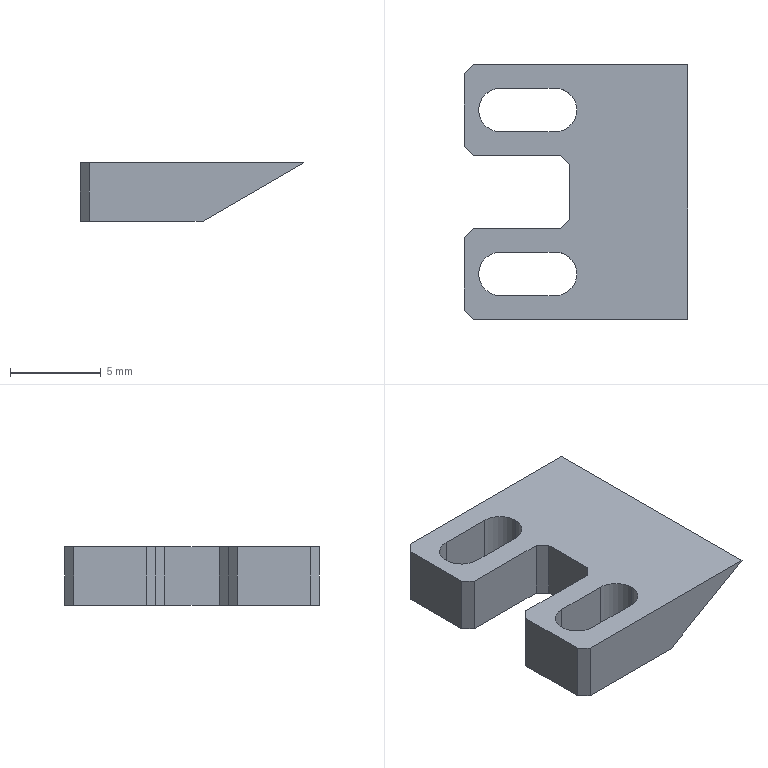NC program | NX | posted with a generic post | part box 12.3 x 14 x 3.2 mm
Whole program:
N10 G17 G21 G94 G90
(FLOOR_WALL , TOOL : D10JING)
N12 T09 M6
N14 G54
N16 G17 G0 G90 X17. Y-8.147 S9500 M3
N18 G43 Z30. H9
N20 Z3.
N22 G94 G1 Z0. F1250.
N24 X14.
N26 X-14.
N28 Y-4.048
N30 X14.
N32 Y0.051
N34 X-14.
N36 Y4.15
N38 X14.
N40 X17.
N42 Z3.
N44 G0 Z30.
N46 M5
(ZLEVEL_PROFILE , TOOL : D6)
N48 T06 M6
N50 G54
N52 G17 G0 G90 X-10.1 Y5.695 S9500 M3
N54 G43 Z30. H6
N56 Z1.5
N58 G94 G1 Y6.082 Z1.48 F1000.
N60 X-9.903 Y6.82 Z1.44
N62 X-9.534 Y7.488 Z1.4
N64 X-9.192 Y7.842 Z1.374
N66 X-8.692 Y8.342 Z1.337
N68 X-8.386 Y8.648 Z1.314
N70 X-7.698 Y9.042 Z1.273
N72 X-6.932 Y9.25 Z1.231
N74 X-2.068 Z0.976
N76 X-1.302 Y9.042 Z0.935
N78 X-0.614 Y8.648 Z0.893
N80 X-0.308 Y8.342 Z0.87
N82 X-0.001 Y8.033 Z0.847
N84 X0.614 Y8.648 Z0.802
N86 X1.302 Y9.042 Z0.76
N88 X2.068 Y9.25 Z0.719
N90 X6.932 Z0.464
N92 X7.672 Y9.052 Z0.424
N94 X8.341 Y8.681 Z0.384
N96 X8.692 Y8.342 Z0.358
N98 X9.192 Y7.842 Z0.321
N100 X9.498 Y7.536 Z0.298
N102 X9.892 Y6.848 Z0.257
N104 X10.1 Y6.082 Z0.215
N106 Y-1.362 Z-0.175
N108 X10.107 Y-1.798 Z-0.198
N110 X9.82 Y-2.783 Z-0.252
N112 X9.234 Y-3.625 Z-0.305
N114 X8.411 Y-4.237 Z-0.359
N116 X7.436 Y-4.555 Z-0.413
N118 X7. Y-4.562 Z-0.436
N120 X-7. F2500.
N122 G2 X-10.1 Y-1.362 R3.181
N124 G1 Y5.65
N126 G2 X-9.192 Y7.842 R3.1
N128 G1 X-8.692 Y8.342
N130 G2 X-6.5 Y9.25 R3.1
N132 G1 X-2.5
N134 G2 X-0.308 Y8.342 R3.1
N136 G1 X-0.001 Y8.033
N138 X0.308 Y8.342
N140 G2 X2.5 Y9.25 R3.1
N142 G1 X6.5
N144 G2 X8.692 Y8.342 R3.1
N146 G1 X9.192 Y7.842
N148 G2 X10.1 Y5.65 R3.1
N150 G1 Y-1.362
N152 G2 X7. Y-4.562 R3.15
N154 G1 X-6.67 Y-4.975 Z-0.674
N156 X-6.99 Y-4.984 Z-0.68
N158 X-7.31 Y-4.976 Z-0.685
N160 X-7.645 Y-4.932 Z-0.69
N162 X-7.97 Y-4.838 Z-0.695
N164 X-8.29 Y-4.73 Z-0.7
N166 X-8.591 Y-4.577 Z-0.705
N168 X-8.866 Y-4.388 Z-0.711
N170 X-9.125 Y-4.173 Z-0.716
N172 X-9.342 Y-3.924 Z-0.721
N174 X-9.556 Y-3.671 Z-0.726
N176 X-9.727 Y-3.398 Z-0.731
N178 X-9.87 Y-3.103 Z-0.737
N180 X-9.973 Y-2.806 Z-0.742
N182 X-10.033 Y-2.488 Z-0.747
N184 X-10.075 Y-2.185 Z-0.752
N186 X-10.1 Y-1.877 Z-0.757
N188 Y-1.279 Z-0.768
N190 Y4.664 Z-0.871
N192 Y5.65
N194 G2 X-9.192 Y7.842 R3.1
N196 G1 X-8.692 Y8.342
N198 G2 X-6.5 Y9.25 R3.1
N200 G1 X-2.5
N202 G2 X-0.308 Y8.342 R3.1
N204 G1 X-0.001 Y8.034
N206 X0.308 Y8.342
N208 G2 X2.5 Y9.25 R3.1
N210 G1 X6.5
N212 G2 X8.692 Y8.342 R3.1
N214 G1 X9.192 Y7.842
N216 G2 X10.1 Y5.65 R3.1
N218 G1 Y-2.117
N220 G2 X7.016 Y-5.317 R3.15
N222 G1 X6.719 Y-5.326 Z-0.877
N224 X-6.654 Y-5.73 Z-1.11
N226 X-6.968 Y-5.739 Z-1.115
N228 X-7.282 Y-5.734 Z-1.12
N230 X-7.618 Y-5.693 Z-1.126
N232 X-7.945 Y-5.603 Z-1.131
N234 X-8.265 Y-5.497 Z-1.136
N236 X-8.568 Y-5.347 Z-1.141
N238 X-8.844 Y-5.16 Z-1.146
N240 X-9.105 Y-4.949 Z-1.152
N242 X-9.323 Y-4.702 Z-1.157
N244 X-9.54 Y-4.452 Z-1.162
N246 X-9.713 Y-4.18 Z-1.167
N248 X-9.859 Y-3.888 Z-1.172
N250 X-9.963 Y-3.591 Z-1.177
N252 X-10.028 Y-3.275 Z-1.183
N254 X-10.07 Y-2.972 Z-1.188
N256 X-10.1 Y-2.665 Z-1.193
N258 Y-2.064 Z-1.203
N260 Y3.879 Z-1.307
N262 Y5.65
N264 G2 X-9.192 Y7.842 R3.1
N266 G1 X-8.692 Y8.342
N268 G2 X-6.5 Y9.25 R3.1
N270 G1 X-2.5
N272 G2 X-0.308 Y8.342 R3.1
N274 G1 X0. Y8.034
N276 X0.308 Y8.342
N278 G2 X2.5 Y9.25 R3.1
N280 G1 X6.5
N282 G2 X8.692 Y8.342 R3.1
N284 G1 X9.192 Y7.842
N286 G2 X10.1 Y5.65 R3.1
N288 G1 Y-2.871
N290 G2 X7.038 Y-6.071 R3.154
N292 G1 X6.741 Y-6.08 Z-1.312
N294 X6.443 Y-6.089 Z-1.318
N296 X-6.632 Y-6.485 Z-1.546
N298 X-6.945 Y-6.494 Z-1.551
N300 X-7.257 Y-6.491 Z-1.556
N302 X-7.593 Y-6.453 Z-1.561
N304 X-7.921 Y-6.366 Z-1.566
N306 X-8.084 Y-6.323 Z-1.569
N308 X-8.24 Y-6.262 Z-1.572
N310 X-8.393 Y-6.193 Z-1.574
N312 X-8.531 Y-6.085 Z-1.577
N314 X-8.688 Y-6.023 Z-1.579
N316 X-8.826 Y-5.929 Z-1.582
N318 X-8.958 Y-5.828 Z-1.585
N320 X-9.087 Y-5.721 Z-1.587
N322 X-9.308 Y-5.476 Z-1.592
N324 X-9.526 Y-5.228 Z-1.598
N326 X-9.702 Y-4.957 Z-1.603
N328 X-9.848 Y-4.665 Z-1.608
N330 X-9.956 Y-4.368 Z-1.613
N332 X-10.025 Y-4.054 Z-1.618
N334 X-10.068 Y-3.75 Z-1.624
N336 X-10.1 Y-3.443 Z-1.629
N338 Y-3.143 Z-1.634
N340 Y-2.842 Z-1.639
N342 Y3.101 Z-1.743
N344 Y5.65
N346 G2 X-9.192 Y7.842 R3.1
N348 G1 X-8.692 Y8.342
N350 G2 X-6.5 Y9.25 R3.1
N352 G1 X-2.5
N354 G2 X-0.308 Y8.342 R3.1
N356 G1 X0. Y8.034
N358 X0.308 Y8.342
N360 G2 X2.5 Y9.25 R3.1
N362 G1 X6.5
N364 G2 X8.692 Y8.342 R3.1
N366 G1 X9.192 Y7.842
N368 G2 X10.1 Y5.65 R3.1
N370 G1 Y-3.626
N372 G2 X7.065 Y-6.824 R3.15
N374 G1 X6.768 Y-6.835 Z-1.748
N376 X6.471 Y-6.844 Z-1.753
N378 X-6.604 Y-7.239 Z-1.981
N380 X-6.919 Y-7.248 Z-1.987
N382 X-7.233 Z-1.992
N384 X-7.569 Y-7.212 Z-1.997
N386 X-7.897 Y-7.129 Z-2.002
N388 X-8.06 Y-7.086 Z-2.005
N390 X-8.217 Y-7.027 Z-2.007
N392 X-8.37 Y-6.96 Z-2.01
N394 X-8.509 Y-6.853 Z-2.013
N396 X-8.667 Y-6.792 Z-2.015
N398 X-8.805 Y-6.7 Z-2.018
N400 X-8.939 Y-6.599 Z-2.02
N402 X-9.068 Y-6.492 Z-2.023
N404 X-9.293 Y-6.25 Z-2.028
N406 X-9.512 Y-6.002 Z-2.033
N408 X-9.69 Y-5.733 Z-2.039
N410 X-9.838 Y-5.441 Z-2.044
N412 X-9.948 Y-5.145 Z-2.049
N414 X-10.022 Y-4.832 Z-2.054
N416 X-10.065 Y-4.528 Z-2.059
N418 X-10.099 Y-4.221 Z-2.064
N420 X-10.1 Y-3.921 Z-2.07
N422 Y-3.621 Z-2.075
N424 Y2.322 Z-2.179
N426 Y5.65
N428 G2 X-9.192 Y7.842 R3.1
N430 G1 X-8.692 Y8.342
N432 G2 X-6.5 Y9.25 R3.1
N434 G1 X-2.5
N436 G2 X-0.308 Y8.342 R3.1
N438 G1 X0. Y8.034
N440 X0.308 Y8.342
N442 G2 X2.5 Y9.25 R3.1
N444 G1 X6.5
N446 G2 X8.692 Y8.342 R3.1
N448 G1 X9.192 Y7.842
N450 G2 X10.1 Y5.65 R3.1
N452 G1 Y-4.381
N454 G2 X7.102 Y-7.578 R3.15
N456 G1 X6.804 Y-7.59 Z-2.184
N458 X6.507 Y-7.599 Z-2.189
N460 X-6.568 Y-7.994 Z-2.417
N462 X-6.882 Y-8.003 Z-2.422
N464 X-7.196 Y-8.005 Z-2.428
N466 X-7.532 Y-7.974 Z-2.433
N468 X-7.861 Y-7.894 Z-2.438
N470 X-8.025 Y-7.854 Z-2.441
N472 X-8.183 Y-7.797 Z-2.443
N474 X-8.338 Y-7.731 Z-2.446
N476 X-8.478 Y-7.625 Z-2.448
N478 X-8.777 Y-7.475 Z-2.453
N480 X-9.046 Y-7.275 Z-2.459
N482 X-9.271 Y-7.031 Z-2.464
N484 X-9.493 Y-6.783 Z-2.469
N486 X-9.675 Y-6.515 Z-2.474
N488 X-9.826 Y-6.223 Z-2.479
N490 X-9.939 Y-5.927 Z-2.485
N492 X-10.018 Y-5.614 Z-2.49
N494 X-10.061 Y-5.308 Z-2.495
N496 X-10.099 Y-5. Z-2.5
N498 X-10.1 Y-4.699 Z-2.505
N500 Y-4.399 Z-2.511
N502 Y1.545 Z-2.614
N504 Y5.65
N506 G2 X-9.192 Y7.842 R3.1
N508 G1 X-8.692 Y8.342
N510 G2 X-6.5 Y9.25 R3.1
N512 G1 X-2.5
N514 G2 X-0.308 Y8.342 R3.1
N516 G1 X0. Y8.034
N518 X0.308 Y8.342
N520 G2 X2.5 Y9.25 R3.1
N522 G1 X6.5
N524 G2 X8.692 Y8.342 R3.1
N526 G1 X9.192 Y7.842
N528 G2 X10.1 Y5.65 R3.1
N530 G1 Y-5.136
N532 G2 X7.149 Y-8.33 R3.15
N534 G1 X6.852 Y-8.344 Z-2.619
N536 X6.555 Y-8.353 Z-2.625
N538 X-6.52 Y-8.749 Z-2.853
N540 X-6.825 Y-8.758 Z-2.858
N542 X-7.13 Y-8.764 Z-2.863
N544 X-7.468 Y-8.739 Z-2.868
N546 X-7.802 Y-8.677 Z-2.874
N548 X-8.124 Y-8.576 Z-2.879
N550 X-8.436 Y-8.443 Z-2.884
N552 X-8.727 Y-8.276 Z-2.889
N554 X-8.998 Y-8.077 Z-2.894
N556 X-9.241 Y-7.851 Z-2.9
N558 X-9.459 Y-7.599 Z-2.905
N560 X-9.642 Y-7.331 Z-2.91
N562 X-9.79 Y-7.036 Z-2.915
N564 X-9.903 Y-6.739 Z-2.92
N566 X-10.005 Y-6.438 Z-2.926
N568 X-10.052 Y-6.129 Z-2.931
N570 X-10.092 Y-5.819 Z-2.936
N572 X-10.1 Y-5.52 Z-2.941
N574 Y-5.22 Z-2.946
N576 Y-4.625 Z-2.957
N578 Y0.724 Z-3.05
N580 Y5.65
N582 G2 X-9.192 Y7.842 R3.1
N584 G1 X-8.692 Y8.342
N586 G2 X-6.5 Y9.25 R3.1
N588 G1 X-2.5
N590 G2 X-0.308 Y8.342 R3.1
N592 G1 X0. Y8.034
N594 X0.308 Y8.342
N596 G2 X2.5 Y9.25 R3.1
N598 G1 X6.5
N600 G2 X8.692 Y8.342 R3.1
N602 G1 X9.192 Y7.842
N604 G2 X10.1 Y5.65 R3.1
N606 G1 Y-5.89
N608 G2 X7. Y-9.09 R3.15
N610 G1 X-7.
N612 G2 X-10.1 Y-5.89 R3.194
N614 G1 Y0.724
N616 Z-1.55
N618 G0 Z30.
N620 M5
(ZLEVEL_PROFILE_COPY_1_COPY , TOOL : D2)
N622 T02 M6
N624 G54
N626 G17 G0 G90 X-4.3 Y1.46 S9500 M3
N628 G43 Z30. H2
N630 Z1.
N632 G94 G1 Y4.15 Z0.859 F1000.
N634 Y4.264 Z0.853
N636 X-4.504 Y4.38 Z0.841
N638 X-4.602 Y4.322 Z0.835
N640 X-4.7 Y4.264 Z0.829
N642 Y1.036 Z0.66
N644 X-4.604 Y0.945 Z0.653
N646 X-4.377 Y0.956 Z0.641
N648 X-4.3 Y1.036 Z0.635
N650 Y4.15 Z0.472
N652 Y4.264 Z0.466
N654 X-4.504 Y4.38 Z0.454
N656 X-4.602 Y4.322 Z0.448
N658 X-4.7 Y4.264 Z0.442
N660 Y1.036 Z0.272
N662 X-4.604 Y0.945 Z0.265
N664 X-4.377 Y0.956 Z0.254
N666 X-4.3 Y1.036 Z0.248
N668 Y4.15 Z0.085
N670 Y4.264 Z0.079
N672 X-4.504 Y4.38 Z0.066
N674 X-4.602 Y4.322 Z0.06
N676 X-4.7 Y4.264 Z0.054
N678 Y1.036 Z-0.115
N680 X-4.604 Y0.945 Z-0.122
N682 X-4.377 Y0.956 Z-0.134
N684 X-4.3 Y1.036 Z-0.14
N686 Y1.15 Z-0.145
N688 Y4.15 F2500.
N690 G3 X-4.5 Y4.35 R0.2
N692 X-4.7 Y4.15 R0.2
N694 G1 Y1.15
N696 G3 X-4.5 Y0.95 R0.2
N698 X-4.3 Y1.15 R0.2
N700 G1 Y4.041 Z-0.223
N702 X-4.309 Y4.21 Z-0.227
N704 X-4.42 Y4.333 Z-0.232
N706 X-4.585 Y4.331 Z-0.236
N708 X-4.692 Y4.206 Z-0.241
N710 X-4.7 Y4.037 Z-0.245
N712 Y2.336 Z-0.291
N714 Y1.15
N716 G3 X-4.5 Y0.95 R0.2
N718 X-4.3 Y1.15 R0.2
N720 G1 Y4.041 Z-0.368
N722 X-4.309 Y4.21 Z-0.373
N724 X-4.42 Y4.333 Z-0.377
N726 X-4.585 Y4.331 Z-0.382
N728 X-4.692 Y4.206 Z-0.386
N730 X-4.7 Y4.037 Z-0.391
N732 Y2.336 Z-0.436
N734 Y1.15
N736 G3 X-4.5 Y0.95 R0.2
N738 X-4.3 Y1.15 R0.2
N740 G1 Y4.041 Z-0.514
N742 X-4.309 Y4.21 Z-0.518
N744 X-4.42 Y4.333 Z-0.523
N746 X-4.585 Y4.331 Z-0.527
N748 X-4.692 Y4.206 Z-0.532
N750 X-4.7 Y4.037 Z-0.536
N752 Y2.336 Z-0.582
N754 Y1.15
N756 G3 X-4.5 Y0.95 R0.2
N758 X-4.3 Y1.15 R0.2
N760 G1 Y4.041 Z-0.659
N762 X-4.309 Y4.21 Z-0.664
N764 X-4.42 Y4.333 Z-0.668
N766 X-4.585 Y4.331 Z-0.673
N768 X-4.692 Y4.206 Z-0.677
N770 X-4.7 Y4.037 Z-0.682
N772 Y2.336 Z-0.727
N774 Y1.15
N776 G3 X-4.5 Y0.95 R0.2
N778 X-4.3 Y1.15 R0.2
N780 G1 Y4.041 Z-0.805
N782 X-4.309 Y4.21 Z-0.809
N784 X-4.42 Y4.333 Z-0.814
N786 X-4.585 Y4.331 Z-0.818
N788 X-4.692 Y4.206 Z-0.823
N790 X-4.7 Y4.037 Z-0.827
N792 Y2.336 Z-0.873
N794 Y1.15
N796 G3 X-4.5 Y0.95 R0.2
N798 X-4.3 Y1.15 R0.2
N800 G1 Y4.041 Z-0.95
N802 X-4.309 Y4.21 Z-0.955
N804 X-4.42 Y4.333 Z-0.959
N806 X-4.585 Y4.331 Z-0.964
N808 X-4.692 Y4.206 Z-0.968
N810 X-4.7 Y4.037 Z-0.973
N812 Y2.336 Z-1.018
N814 Y1.15
N816 G3 X-4.5 Y0.95 R0.2
N818 X-4.3 Y1.15 R0.2
N820 G1 Y4.041 Z-1.095
N822 X-4.309 Y4.21 Z-1.1
N824 X-4.42 Y4.333 Z-1.105
N826 X-4.585 Y4.331 Z-1.109
N828 X-4.692 Y4.206 Z-1.114
N830 X-4.7 Y4.037 Z-1.118
N832 Y2.336 Z-1.164
N834 Y1.15
N836 G3 X-4.5 Y0.95 R0.2
N838 X-4.3 Y1.15 R0.2
N840 G1 Y4.041 Z-1.241
N842 X-4.309 Y4.21 Z-1.245
N844 X-4.42 Y4.333 Z-1.25
N846 X-4.585 Y4.331 Z-1.255
N848 X-4.692 Y4.206 Z-1.259
N850 X-4.7 Y4.037 Z-1.264
N852 Y2.336 Z-1.309
N854 Y1.15
N856 G3 X-4.5 Y0.95 R0.2
N858 X-4.3 Y1.15 R0.2
N860 G1 Y4.041 Z-1.386
N862 X-4.309 Y4.21 Z-1.391
N864 X-4.42 Y4.333 Z-1.395
N866 X-4.585 Y4.331 Z-1.4
N868 X-4.692 Y4.206 Z-1.405
N870 X-4.7 Y4.037 Z-1.409
N872 Y2.336 Z-1.455
N874 Y1.15
N876 G3 X-4.5 Y0.95 R0.2
N878 X-4.3 Y1.15 R0.2
N880 G1 Y4.041 Z-1.532
N882 X-4.309 Y4.21 Z-1.536
N884 X-4.42 Y4.333 Z-1.541
N886 X-4.585 Y4.331 Z-1.545
N888 X-4.692 Y4.206 Z-1.55
N890 X-4.7 Y4.037 Z-1.555
N892 Y2.336 Z-1.6
N894 Y1.15
N896 G3 X-4.5 Y0.95 R0.2
N898 X-4.3 Y1.15 R0.2
N900 G1 Y4.041 Z-1.677
N902 X-4.309 Y4.21 Z-1.682
N904 X-4.42 Y4.333 Z-1.686
N906 X-4.585 Y4.331 Z-1.691
N908 X-4.692 Y4.206 Z-1.695
N910 X-4.7 Y4.037 Z-1.7
N912 Y2.336 Z-1.745
N914 Y1.15
N916 G3 X-4.5 Y0.95 R0.2
N918 X-4.3 Y1.15 R0.2
N920 G1 Y4.041 Z-1.823
N922 X-4.309 Y4.21 Z-1.827
N924 X-4.42 Y4.333 Z-1.832
N926 X-4.585 Y4.331 Z-1.836
N928 X-4.692 Y4.206 Z-1.841
N930 X-4.7 Y4.037 Z-1.845
N932 Y2.336 Z-1.891
N934 Y1.15
N936 G3 X-4.5 Y0.95 R0.2
N938 X-4.3 Y1.15 R0.2
N940 G1 Y4.041 Z-1.968
N942 X-4.309 Y4.21 Z-1.973
N944 X-4.42 Y4.333 Z-1.977
N946 X-4.585 Y4.331 Z-1.982
N948 X-4.692 Y4.206 Z-1.986
N950 X-4.7 Y4.037 Z-1.991
N952 Y2.336 Z-2.036
N954 Y1.15
N956 G3 X-4.5 Y0.95 R0.2
N958 X-4.3 Y1.15 R0.2
N960 G1 Y4.041 Z-2.114
N962 X-4.309 Y4.21 Z-2.118
N964 X-4.42 Y4.333 Z-2.123
N966 X-4.585 Y4.331 Z-2.127
N968 X-4.692 Y4.206 Z-2.132
N970 X-4.7 Y4.037 Z-2.136
N972 Y2.336 Z-2.182
N974 Y1.15
N976 G3 X-4.5 Y0.95 R0.2
N978 X-4.3 Y1.15 R0.2
N980 G1 Y4.041 Z-2.259
N982 X-4.309 Y4.21 Z-2.264
N984 X-4.42 Y4.333 Z-2.268
N986 X-4.585 Y4.331 Z-2.273
N988 X-4.692 Y4.206 Z-2.277
N990 X-4.7 Y4.037 Z-2.282
N992 Y2.336 Z-2.327
N994 Y1.15
N996 G3 X-4.5 Y0.95 R0.2
N998 X-4.3 Y1.15 R0.2
N1000 G1 Y4.041 Z-2.405
N1002 X-4.309 Y4.21 Z-2.409
N1004 X-4.42 Y4.333 Z-2.414
N1006 X-4.585 Y4.331 Z-2.418
N1008 X-4.692 Y4.206 Z-2.423
N1010 X-4.7 Y4.037 Z-2.427
N1012 Y2.336 Z-2.473
N1014 Y1.15
N1016 G3 X-4.5 Y0.95 R0.2
N1018 X-4.3 Y1.15 R0.2
N1020 G1 Y4.041 Z-2.55
N1022 X-4.309 Y4.21 Z-2.555
N1024 X-4.42 Y4.333 Z-2.559
N1026 X-4.585 Y4.331 Z-2.564
N1028 X-4.692 Y4.206 Z-2.568
N1030 X-4.7 Y4.037 Z-2.573
N1032 Y2.336 Z-2.618
N1034 Y1.15
N1036 G3 X-4.5 Y0.95 R0.2
N1038 X-4.3 Y1.15 R0.2
N1040 G1 Y4.041 Z-2.695
N1042 X-4.309 Y4.21 Z-2.7
N1044 X-4.42 Y4.333 Z-2.705
N1046 X-4.585 Y4.331 Z-2.709
N1048 X-4.692 Y4.206 Z-2.714
N1050 X-4.7 Y4.037 Z-2.718
N1052 Y2.336 Z-2.764
N1054 Y1.15
N1056 G3 X-4.5 Y0.95 R0.2
N1058 X-4.3 Y1.15 R0.2
N1060 G1 Y4.041 Z-2.841
N1062 X-4.309 Y4.21 Z-2.845
N1064 X-4.42 Y4.333 Z-2.85
N1066 X-4.585 Y4.331 Z-2.855
N1068 X-4.692 Y4.206 Z-2.859
N1070 X-4.7 Y4.037 Z-2.864
N1072 Y2.336 Z-2.909
N1074 Y1.15
N1076 G3 X-4.5 Y0.95 R0.2
N1078 X-4.3 Y1.15 R0.2
N1080 G1 Y4.041 Z-2.986
N1082 X-4.309 Y4.21 Z-2.991
N1084 X-4.42 Y4.333 Z-2.995
N1086 X-4.585 Y4.331 Z-3.
N1088 X-4.692 Y4.206 Z-3.005
N1090 X-4.7 Y4.037 Z-3.009
N1092 Y2.336 Z-3.055
N1094 Y1.15
N1096 G3 X-4.5 Y0.95 R0.2
N1098 X-4.3 Y1.15 R0.2
N1100 G1 Y4.041 Z-3.132
N1102 X-4.309 Y4.21 Z-3.136
N1104 X-4.42 Y4.333 Z-3.141
N1106 X-4.585 Y4.331 Z-3.145
N1108 X-4.692 Y4.206 Z-3.15
N1110 X-4.7 Y4.037 Z-3.155
N1112 Y2.336 Z-3.2
N1114 Y1.15
N1116 G3 X-4.5 Y0.95 R0.2
N1118 X-4.3 Y1.15 R0.2
N1120 G1 Y4.15
N1122 G3 X-4.5 Y4.35 R0.2
N1124 X-4.7 Y4.15 R0.2
N1126 G1 Y2.336
N1128 Z-2.2
N1130 G0 Z30.
N1132 X4.3 Y3.84
N1134 Z1.
N1136 G1 Y1.036 Z0.853 F1000.
N1138 X4.377 Y0.956 Z0.847
N1140 X4.604 Y0.945 Z0.835
N1142 X4.7 Y1.036 Z0.828
N1144 Y4.264 Z0.659
N1146 X4.504 Y4.38 Z0.647
N1148 X4.3 Y4.264 Z0.635
N1150 Y4.15 Z0.629
N1152 Y1.036 Z0.466
N1154 X4.377 Y0.956 Z0.46
N1156 X4.604 Y0.945 Z0.448
N1158 X4.7 Y1.036 Z0.441
N1160 Y4.264 Z0.272
N1162 X4.504 Y4.38 Z0.26
N1164 X4.3 Y4.264 Z0.248
N1166 Y4.15 Z0.242
N1168 Y1.036 Z0.079
N1170 X4.377 Y0.956 Z0.073
N1172 X4.604 Y0.945 Z0.061
N1174 X4.7 Y1.036 Z0.054
N1176 Y4.264 Z-0.115
N1178 X4.504 Y4.38 Z-0.127
N1180 X4.3 Y4.264 Z-0.14
N1182 Y4.15 Z-0.145
N1184 Y1.15 F2500.
N1186 G3 X4.5 Y0.95 R0.2
N1188 X4.7 Y1.15 R0.2
N1190 G1 Y4.15
N1192 G3 X4.5 Y4.35 R0.2
N1194 X4.3 Y4.15 R0.2
N1196 G1 Y1.259 Z-0.223
N1198 X4.309 Y1.09 Z-0.227
N1200 X4.42 Y0.967 Z-0.232
N1202 X4.585 Y0.969 Z-0.236
N1204 X4.692 Y1.094 Z-0.241
N1206 X4.7 Y1.263 Z-0.245
N1208 Y2.964 Z-0.291
N1210 Y4.15
N1212 G3 X4.5 Y4.35 R0.2
N1214 X4.3 Y4.15 R0.2
N1216 G1 Y1.259 Z-0.368
N1218 X4.309 Y1.09 Z-0.373
N1220 X4.42 Y0.967 Z-0.377
N1222 X4.585 Y0.969 Z-0.382
N1224 X4.692 Y1.094 Z-0.386
N1226 X4.7 Y1.263 Z-0.391
N1228 Y2.964 Z-0.436
N1230 Y4.15
N1232 G3 X4.5 Y4.35 R0.2
N1234 X4.3 Y4.15 R0.2
N1236 G1 Y1.259 Z-0.514
N1238 X4.309 Y1.09 Z-0.518
N1240 X4.42 Y0.967 Z-0.523
N1242 X4.585 Y0.969 Z-0.527
N1244 X4.692 Y1.094 Z-0.532
N1246 X4.7 Y1.263 Z-0.536
N1248 Y2.964 Z-0.582
N1250 Y4.15
N1252 G3 X4.5 Y4.35 R0.2
N1254 X4.3 Y4.15 R0.2
N1256 G1 Y1.259 Z-0.659
N1258 X4.309 Y1.09 Z-0.664
N1260 X4.42 Y0.967 Z-0.668
N1262 X4.585 Y0.969 Z-0.673
N1264 X4.692 Y1.094 Z-0.677
N1266 X4.7 Y1.263 Z-0.682
N1268 Y2.964 Z-0.727
N1270 Y4.15
N1272 G3 X4.5 Y4.35 R0.2
N1274 X4.3 Y4.15 R0.2
N1276 G1 Y1.259 Z-0.805
N1278 X4.309 Y1.09 Z-0.809
N1280 X4.42 Y0.967 Z-0.814
N1282 X4.585 Y0.969 Z-0.818
N1284 X4.692 Y1.094 Z-0.823
N1286 X4.7 Y1.263 Z-0.827
N1288 Y2.964 Z-0.873
N1290 Y4.15
N1292 G3 X4.5 Y4.35 R0.2
N1294 X4.3 Y4.15 R0.2
N1296 G1 Y1.259 Z-0.95
N1298 X4.309 Y1.09 Z-0.955
N1300 X4.42 Y0.967 Z-0.959
N1302 X4.585 Y0.969 Z-0.964
N1304 X4.692 Y1.094 Z-0.968
N1306 X4.7 Y1.263 Z-0.973
N1308 Y2.964 Z-1.018
N1310 Y4.15
N1312 G3 X4.5 Y4.35 R0.2
N1314 X4.3 Y4.15 R0.2
N1316 G1 Y1.259 Z-1.095
N1318 X4.309 Y1.09 Z-1.1
N1320 X4.42 Y0.967 Z-1.105
N1322 X4.585 Y0.969 Z-1.109
N1324 X4.692 Y1.094 Z-1.114
N1326 X4.7 Y1.263 Z-1.118
N1328 Y2.964 Z-1.164
N1330 Y4.15
N1332 G3 X4.5 Y4.35 R0.2
N1334 X4.3 Y4.15 R0.2
N1336 G1 Y1.259 Z-1.241
N1338 X4.309 Y1.09 Z-1.245
N1340 X4.42 Y0.967 Z-1.25
N1342 X4.585 Y0.969 Z-1.255
N1344 X4.692 Y1.094 Z-1.259
N1346 X4.7 Y1.263 Z-1.264
N1348 Y2.964 Z-1.309
N1350 Y4.15
N1352 G3 X4.5 Y4.35 R0.2
N1354 X4.3 Y4.15 R0.2
N1356 G1 Y1.259 Z-1.386
N1358 X4.309 Y1.09 Z-1.391
N1360 X4.42 Y0.967 Z-1.395
N1362 X4.585 Y0.969 Z-1.4
N1364 X4.692 Y1.094 Z-1.405
N1366 X4.7 Y1.263 Z-1.409
N1368 Y2.964 Z-1.455
N1370 Y4.15
N1372 G3 X4.5 Y4.35 R0.2
N1374 X4.3 Y4.15 R0.2
N1376 G1 Y1.259 Z-1.532
N1378 X4.309 Y1.09 Z-1.536
N1380 X4.42 Y0.967 Z-1.541
N1382 X4.585 Y0.969 Z-1.545
N1384 X4.692 Y1.094 Z-1.55
N1386 X4.7 Y1.263 Z-1.555
N1388 Y2.964 Z-1.6
N1390 Y4.15
N1392 G3 X4.5 Y4.35 R0.2
N1394 X4.3 Y4.15 R0.2
N1396 G1 Y1.259 Z-1.677
N1398 X4.309 Y1.09 Z-1.682
N1400 X4.42 Y0.967 Z-1.686
N1402 X4.585 Y0.969 Z-1.691
N1404 X4.692 Y1.094 Z-1.695
N1406 X4.7 Y1.263 Z-1.7
N1408 Y2.964 Z-1.745
N1410 Y4.15
N1412 G3 X4.5 Y4.35 R0.2
N1414 X4.3 Y4.15 R0.2
N1416 G1 Y1.259 Z-1.823
N1418 X4.309 Y1.09 Z-1.827
N1420 X4.42 Y0.967 Z-1.832
N1422 X4.585 Y0.969 Z-1.836
N1424 X4.692 Y1.094 Z-1.841
N1426 X4.7 Y1.263 Z-1.845
N1428 Y2.964 Z-1.891
N1430 Y4.15
N1432 G3 X4.5 Y4.35 R0.2
N1434 X4.3 Y4.15 R0.2
N1436 G1 Y1.259 Z-1.968
N1438 X4.309 Y1.09 Z-1.973
N1440 X4.42 Y0.967 Z-1.977
N1442 X4.585 Y0.969 Z-1.982
N1444 X4.692 Y1.094 Z-1.986
N1446 X4.7 Y1.263 Z-1.991
N1448 Y2.964 Z-2.036
N1450 Y4.15
N1452 G3 X4.5 Y4.35 R0.2
N1454 X4.3 Y4.15 R0.2
N1456 G1 Y1.259 Z-2.114
N1458 X4.309 Y1.09 Z-2.118
N1460 X4.42 Y0.967 Z-2.123
N1462 X4.585 Y0.969 Z-2.127
N1464 X4.692 Y1.094 Z-2.132
N1466 X4.7 Y1.263 Z-2.136
N1468 Y2.964 Z-2.182
N1470 Y4.15
N1472 G3 X4.5 Y4.35 R0.2
N1474 X4.3 Y4.15 R0.2
N1476 G1 Y1.259 Z-2.259
N1478 X4.309 Y1.09 Z-2.264
N1480 X4.42 Y0.967 Z-2.268
N1482 X4.585 Y0.969 Z-2.273
N1484 X4.692 Y1.094 Z-2.277
N1486 X4.7 Y1.263 Z-2.282
N1488 Y2.964 Z-2.327
N1490 Y4.15
N1492 G3 X4.5 Y4.35 R0.2
N1494 X4.3 Y4.15 R0.2
N1496 G1 Y1.259 Z-2.405
N1498 X4.309 Y1.09 Z-2.409
N1500 X4.42 Y0.967 Z-2.414
N1502 X4.585 Y0.969 Z-2.418
N1504 X4.692 Y1.094 Z-2.423
N1506 X4.7 Y1.263 Z-2.427
N1508 Y2.964 Z-2.473
N1510 Y4.15
N1512 G3 X4.5 Y4.35 R0.2
N1514 X4.3 Y4.15 R0.2
N1516 G1 Y1.259 Z-2.55
N1518 X4.309 Y1.09 Z-2.555
N1520 X4.42 Y0.967 Z-2.559
N1522 X4.585 Y0.969 Z-2.564
N1524 X4.692 Y1.094 Z-2.568
N1526 X4.7 Y1.263 Z-2.573
N1528 Y2.964 Z-2.618
N1530 Y4.15
N1532 G3 X4.5 Y4.35 R0.2
N1534 X4.3 Y4.15 R0.2
N1536 G1 Y1.259 Z-2.695
N1538 X4.309 Y1.09 Z-2.7
N1540 X4.42 Y0.967 Z-2.705
N1542 X4.585 Y0.969 Z-2.709
N1544 X4.692 Y1.094 Z-2.714
N1546 X4.7 Y1.263 Z-2.718
N1548 Y2.964 Z-2.764
N1550 Y4.15
N1552 G3 X4.5 Y4.35 R0.2
N1554 X4.3 Y4.15 R0.2
N1556 G1 Y1.259 Z-2.841
N1558 X4.309 Y1.09 Z-2.845
N1560 X4.42 Y0.967 Z-2.85
N1562 X4.585 Y0.969 Z-2.855
N1564 X4.692 Y1.094 Z-2.859
N1566 X4.7 Y1.263 Z-2.864
N1568 Y2.964 Z-2.909
N1570 Y4.15
N1572 G3 X4.5 Y4.35 R0.2
N1574 X4.3 Y4.15 R0.2
N1576 G1 Y1.259 Z-2.986
N1578 X4.309 Y1.09 Z-2.991
N1580 X4.42 Y0.967 Z-2.995
N1582 X4.585 Y0.969 Z-3.
N1584 X4.692 Y1.094 Z-3.005
N1586 X4.7 Y1.263 Z-3.009
N1588 Y2.964 Z-3.055
N1590 Y4.15
N1592 G3 X4.5 Y4.35 R0.2
N1594 X4.3 Y4.15 R0.2
N1596 G1 Y1.259 Z-3.132
N1598 X4.309 Y1.09 Z-3.136
N1600 X4.42 Y0.967 Z-3.141
N1602 X4.585 Y0.969 Z-3.145
N1604 X4.692 Y1.094 Z-3.15
N1606 X4.7 Y1.263 Z-3.155
N1608 Y2.964 Z-3.2
N1610 Y4.15
N1612 G3 X4.5 Y4.35 R0.2
N1614 X4.3 Y4.15 R0.2
N1616 G1 Y1.15
N1618 G3 X4.5 Y0.95 R0.2
N1620 X4.7 Y1.15 R0.2
N1622 G1 Y2.964
N1624 Z-2.2
N1626 G0 Z30.
N1628 M5
(ZLEVEL_PROFILE_1 , TOOL : D2R0.5)
N1630 T05 M6
N1632 G54
N1634 G17 G0 G90 X7.793 Y-1.664 S9500 M3
N1636 G43 Z30. H5
N1638 Z2.96
N1640 G94 G1 Z-0.04 F1000.
N1642 X7.646 Y-1.411
N1644 G3 X7.473 Y-1.311 R0.2
N1646 G1 X-7.473 F2500.
N1648 Y-1.345 Z-0.06
N1650 Y-1.38 Z-0.08
N1652 X-7.
N1654 X7.
N1656 X7.474
N1658 Y-1.415 Z-0.1
N1660 Y-1.449 Z-0.12
N1662 X7.
N1664 X-7.
N1666 X-7.474
N1668 Y-1.484 Z-0.14
N1670 Y-1.518 Z-0.16
N1672 X-7. Y-1.519
N1674 X7.
N1676 X7.474 Y-1.518
N1678 X7.475 Y-1.553 Z-0.18
N1680 Y-1.588 Z-0.2
N1682 X7.
N1684 X-7.
N1686 X-7.475
N1688 Y-1.622 Z-0.22
N1690 Y-1.657 Z-0.24
N1692 X-7.
N1694 X7.
N1696 X7.475
N1698 Y-1.692 Z-0.26
N1700 X7.476 Y-1.726 Z-0.28
N1702 X7.
N1704 X-7.
N1706 X-7.476
N1708 Y-1.761 Z-0.3
N1710 Y-1.796 Z-0.32
N1712 X-7.
N1714 X7.
N1716 X7.476
N1718 Y-1.83 Z-0.34
N1720 Y-1.865 Z-0.36
N1722 X7.
N1724 X-7.
N1726 X-7.476
N1728 X-7.477 Y-1.9 Z-0.38
N1730 Y-1.934 Z-0.4
N1732 X-7.
N1734 X7.
N1736 X7.477
N1738 Y-1.969 Z-0.42
N1740 Y-2.003 Z-0.44
N1742 X7. Y-2.004
N1744 X-7.
N1746 X-7.477 Y-2.003
N1748 X-7.478 Y-2.038 Z-0.46
N1750 Y-2.073 Z-0.48
N1752 X-7.
N1754 X7.
N1756 X7.478
N1758 Y-2.107 Z-0.5
N1760 Y-2.142 Z-0.52
N1762 X7.
N1764 X-7.
N1766 X-7.478
N1768 X-7.479 Y-2.177 Z-0.54
N1770 Y-2.211 Z-0.56
N1772 X-7.
N1774 X7.
N1776 X7.479
N1778 Y-2.246 Z-0.58
N1780 Y-2.281 Z-0.6
N1782 X7.
N1784 X-7.
N1786 X-7.479
N1788 Y-2.315 Z-0.62
N1790 X-7.48 Y-2.35 Z-0.64
N1792 X-7.
N1794 X7.
N1796 X7.48
N1798 Y-2.385 Z-0.66
N1800 Y-2.419 Z-0.68
N1802 X7.
N1804 X-7.
N1806 X-7.48
N1808 Y-2.454 Z-0.7
N1810 X-7.481 Y-2.488 Z-0.72
N1812 X-7.
N1814 X7.
N1816 X7.481
N1818 Y-2.523 Z-0.74
N1820 Y-2.558 Z-0.76
N1822 X7.
N1824 X-7.
N1826 X-7.481
N1828 Y-2.592 Z-0.78
N1830 Y-2.627 Z-0.8
N1832 X-7.
N1834 X7.
N1836 X7.481
N1838 X7.482 Y-2.662 Z-0.82
N1840 Y-2.696 Z-0.84
N1842 X7.
N1844 X-7.
N1846 X-7.482
N1848 Y-2.731 Z-0.86
N1850 Y-2.766 Z-0.88
N1852 X-7.
N1854 X7.
N1856 X7.482
N1858 Y-2.8 Z-0.9
N1860 Y-2.835 Z-0.92
N1862 X7.
N1864 X-7.
N1866 X-7.482
N1868 Y-2.87 Z-0.94
N1870 X-7.483 Y-2.904 Z-0.96
N1872 X-7.
N1874 X7.
N1876 X7.483
N1878 Y-2.939 Z-0.98
N1880 Y-2.973 Z-1.
N1882 X7.
N1884 X-7.
N1886 X-7.483
N1888 Y-3.008 Z-1.02
N1890 Y-3.043 Z-1.04
N1892 X-7.
N1894 X7.
N1896 X7.483
N1898 Y-3.077 Z-1.06
N1900 Y-3.112 Z-1.08
N1902 X7.
N1904 X-7.
N1906 X-7.483
N1908 Y-3.147 Z-1.1
N1910 Y-3.181 Z-1.12
N1912 X-7.
N1914 X7.
N1916 X7.483
N1918 X7.484 Y-3.216 Z-1.14
N1920 Y-3.251 Z-1.16
N1922 X7.
N1924 X-7.
N1926 X-7.484
N1928 Y-3.285 Z-1.18
N1930 Y-3.32 Z-1.2
N1932 X-7.
N1934 X7.
N1936 X7.484
N1938 Y-3.355 Z-1.22
N1940 Y-3.389 Z-1.24
N1942 X7.
N1944 X-7.
N1946 X-7.484
N1948 Y-3.424 Z-1.26
N1950 Y-3.458 Z-1.28
N1952 X-7.
N1954 X7.
N1956 X7.484
N1958 Y-3.493 Z-1.3
N1960 Y-3.528 Z-1.32
N1962 X7.
N1964 X-7.
N1966 X-7.484
N1968 Y-3.562 Z-1.34
N1970 X-7.485 Y-3.597 Z-1.36
N1972 X-7.
N1974 X7.
N1976 X7.485
N1978 Y-3.632 Z-1.38
N1980 Y-3.666 Z-1.4
N1982 X7.
N1984 X-7.
N1986 X-7.485
N1988 Y-3.701 Z-1.42
N1990 Y-3.736 Z-1.44
N1992 X-7.
N1994 X7.
N1996 X7.485
N1998 Y-3.77 Z-1.46
N2000 Y-3.805 Z-1.48
N2002 X7.
N2004 X-7.
N2006 X-7.485
N2008 Y-3.839 Z-1.5
N2010 Y-3.874 Z-1.52
N2012 X-7.
N2014 X7.
N2016 X7.485
N2018 Y-3.909 Z-1.54
N2020 Y-3.943 Z-1.56
N2022 X7.
N2024 X-7.
N2026 X-7.485
N2028 X-7.486 Y-3.978 Z-1.58
N2030 Y-4.013 Z-1.6
N2032 X-7.
N2034 X7.
N2036 X7.486
N2038 Y-4.047 Z-1.62
N2040 Y-4.082 Z-1.64
N2042 X7.
N2044 X-7.
N2046 X-7.486
N2048 Y-4.117 Z-1.66
N2050 Y-4.151 Z-1.68
N2052 X-7.
N2054 X7.
N2056 X7.486
N2058 Y-4.186 Z-1.7
N2060 Y-4.221 Z-1.72
N2062 X7.
N2064 X-7.
N2066 X-7.486
N2068 Y-4.255 Z-1.74
N2070 Y-4.29 Z-1.76
N2072 X-7.
N2074 X7.
N2076 X7.486
N2078 X7.485 Y-4.324 Z-1.78
N2080 Y-4.359 Z-1.8
N2082 X7.
N2084 X-7.
N2086 X-7.485
N2088 Y-4.394 Z-1.82
N2090 Y-4.428 Z-1.84
N2092 X-7.
N2094 X7.
N2096 X7.485
N2098 Y-4.463 Z-1.86
N2100 Y-4.498 Z-1.88
N2102 X7.
N2104 X-7.
N2106 X-7.485
N2108 Y-4.532 Z-1.9
N2110 Y-4.567 Z-1.92
N2112 X-7.
N2114 X7.
N2116 X7.485
N2118 Y-4.602 Z-1.94
N2120 Y-4.636 Z-1.96
N2122 X7.
N2124 X-7.
N2126 X-7.485
N2128 X-7.484 Y-4.671 Z-1.98
N2130 Y-4.706 Z-2.
N2132 X-7.
N2134 X7.
N2136 X7.484
N2138 Y-4.74 Z-2.02
N2140 Y-4.775 Z-2.04
N2142 X7.
N2144 X-7.
N2146 X-7.484
N2148 Y-4.809 Z-2.06
N2150 Y-4.844 Z-2.08
N2152 X-7.
N2154 X7.
N2156 X7.484
N2158 Y-4.879 Z-2.1
N2160 Y-4.913 Z-2.12
N2162 X7.
N2164 X-7.
N2166 X-7.484
N2168 Y-4.948 Z-2.14
N2170 Y-4.983 Z-2.16
N2172 X-7.
N2174 X7.
N2176 X7.484
N2178 X7.483 Y-5.017 Z-2.18
N2180 Y-5.052 Z-2.2
N2182 X7.
N2184 X-7.
N2186 X-7.484
N2188 X-7.483 Y-5.087 Z-2.22
N2190 Y-5.121 Z-2.24
N2192 X-7.
N2194 X7.
N2196 X7.483
N2198 Y-5.156 Z-2.26
N2200 Y-5.19 Z-2.28
N2202 X7.
N2204 X-7.
N2206 X-7.483
N2208 Y-5.225 Z-2.3
N2210 Y-5.26 Z-2.32
N2212 X-7.
N2214 X7.
N2216 X7.483
N2218 Y-5.294 Z-2.34
N2220 Y-5.329 Z-2.36
N2222 X7.
N2224 X-7.
N2226 X-7.483
N2228 Y-5.364 Z-2.38
N2230 Y-5.398 Z-2.4
N2232 X-7.
N2234 X7.
N2236 X7.483
N2238 X7.482 Y-5.433 Z-2.42
N2240 Y-5.468 Z-2.44
N2242 X7.
N2244 X-7.
N2246 X-7.482
N2248 Y-5.502 Z-2.46
N2250 Y-5.537 Z-2.48
N2252 X-7.
N2254 X7.
N2256 X7.482
N2258 Y-5.572 Z-2.5
N2260 Y-5.606 Z-2.52
N2262 X7.
N2264 X-7.
N2266 X-7.481
N2268 Y-5.641 Z-2.54
N2270 Y-5.675 Z-2.56
N2272 X-7.
N2274 X7.
N2276 X7.481
N2278 Y-5.71 Z-2.58
N2280 Y-5.745 Z-2.6
N2282 X7.
N2284 X-7.
N2286 X-7.481
N2288 X-7.48 Y-5.779 Z-2.62
N2290 Y-5.814 Z-2.64
N2292 X-7.
N2294 X7.
N2296 X7.48
N2298 Y-5.849 Z-2.66
N2300 Y-5.883 Z-2.68
N2302 X7.
N2304 X-7.
N2306 X-7.48
N2308 Y-5.918 Z-2.7
N2310 X-7.479 Y-5.953 Z-2.72
N2312 X-7.
N2314 X7.
N2316 X7.479
N2318 Y-5.987 Z-2.74
N2320 Y-6.022 Z-2.76
N2322 X7.
N2324 X-7.
N2326 X-7.479
N2328 Y-6.057 Z-2.78
N2330 Y-6.091 Z-2.8
N2332 X-7.
N2334 X7.
N2336 X7.479
N2338 X7.478 Y-6.126 Z-2.82
N2340 Y-6.16 Z-2.84
N2342 X7.
N2344 X-7.
N2346 X-7.478
N2348 Y-6.195 Z-2.86
N2350 Y-6.23 Z-2.88
N2352 X-7.
N2354 X7.
N2356 X7.477
N2358 Y-6.264 Z-2.9
N2360 Y-6.299 Z-2.92
N2362 X7.
N2364 X-7.
N2366 X-7.477
N2368 Y-6.334 Z-2.94
N2370 Y-6.368 Z-2.96
N2372 X-7.
N2374 X7.
N2376 X7.477
N2378 X7.476 Y-6.403 Z-2.98
N2380 Y-6.437 Z-3.
N2382 X7. Y-6.438
N2384 X-7.
N2386 X-7.476 Y-6.437
N2388 Y-6.472 Z-3.02
N2390 Y-6.507 Z-3.04
N2392 X-7.
N2394 X7.
N2396 X7.476
N2398 Y-6.541 Z-3.06
N2400 X7.475 Y-6.576 Z-3.08
N2402 X7.
N2404 X-7.
N2406 X-7.475
N2408 Y-6.611 Z-3.1
N2410 Y-6.645 Z-3.12
N2412 X-7.
N2414 X7.
N2416 X7.475
N2418 Y-6.68 Z-3.14
N2420 Y-6.715 Z-3.16
N2422 X7.
N2424 X-7.
N2426 X-7.474
N2428 Y-6.749 Z-3.18
N2430 Y-6.78 Z-3.2
N2432 X-7.
N2434 X7.
N2436 X7.474
N2438 Y-6.819 Z-3.22
N2440 Y-6.853 Z-3.24
N2442 X7.
N2444 X-7.
N2446 X-7.474
N2448 X-7.473 Y-6.888 Z-3.26
N2450 Y-6.922 Z-3.28
N2452 X7.473
N2454 Y-6.957 Z-3.3
N2456 Y-6.992 Z-3.32
N2458 X-7.473
N2460 X-7.472 Y-7.026 Z-3.34
N2462 Y-7.061 Z-3.36
N2464 X7.472
N2466 Y-7.096 Z-3.38
N2468 Y-7.13 Z-3.4
N2470 X-7.472
N2472 X-7.471 Y-7.165 Z-3.42
N2474 Y-7.199 Z-3.44
N2476 X7.471
N2478 X7.414 Y-7.234 Z-3.46
N2480 X7.357 Y-7.266 Z-3.48
N2482 X7.289 Y-7.269
N2484 X-7.289
N2486 X-7.357 Y-7.266
N2488 G3 X-7.534 Y-7.359 R0.2
N2490 G1 X-7.711 Y-7.64
N2492 Z-0.48
N2494 G0 Z30.
N2496 M5
N2498 M2